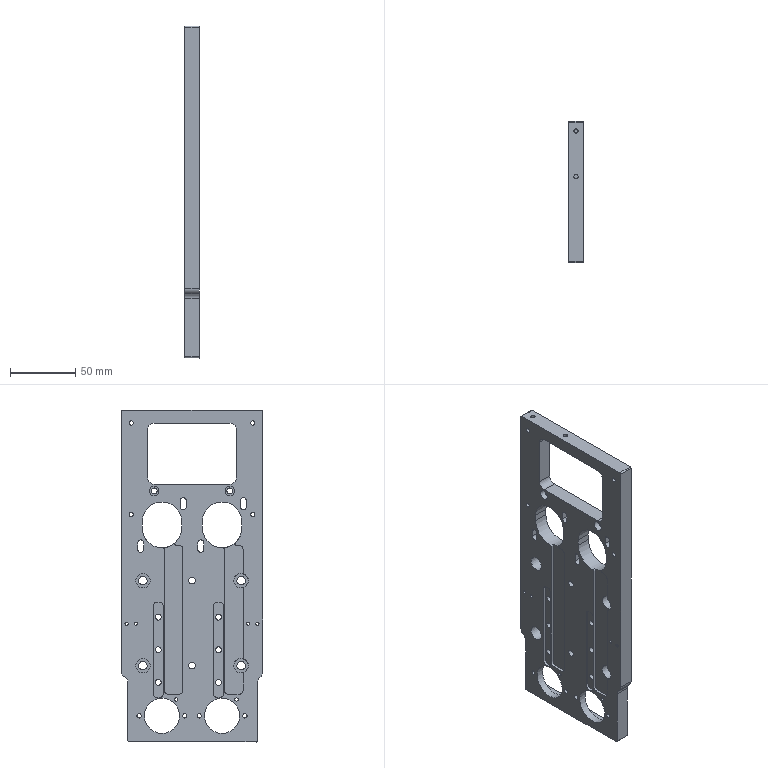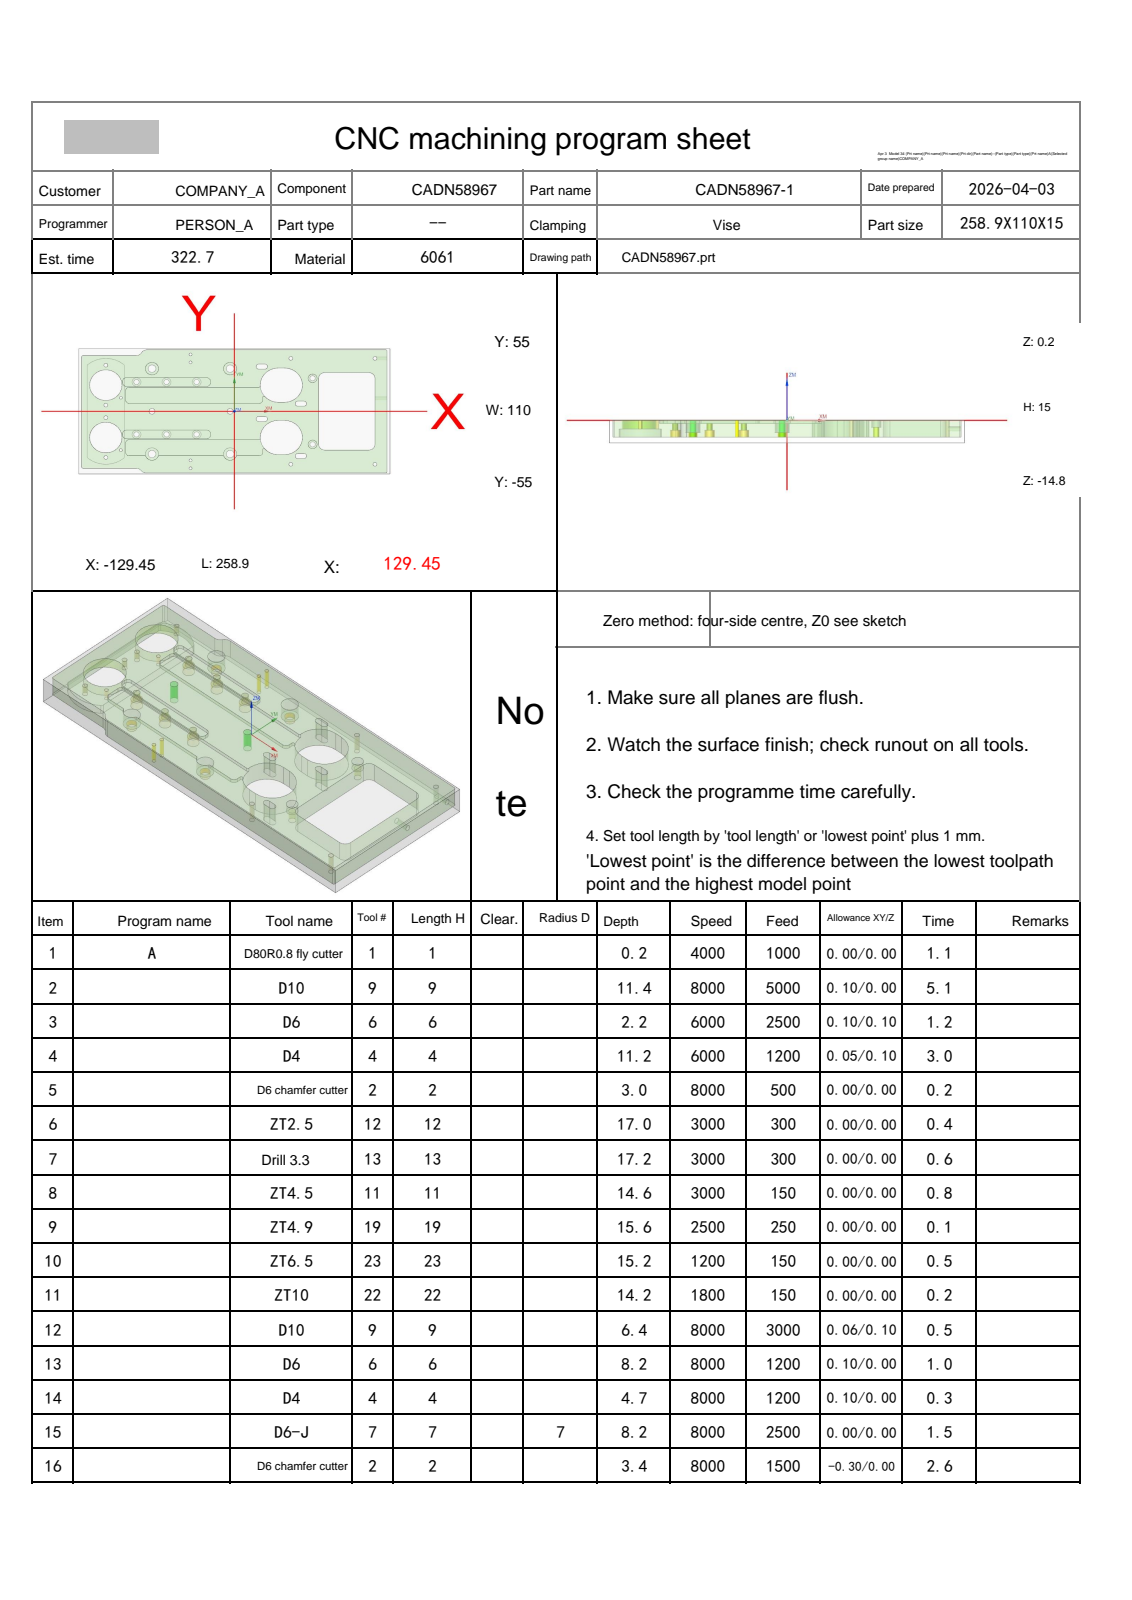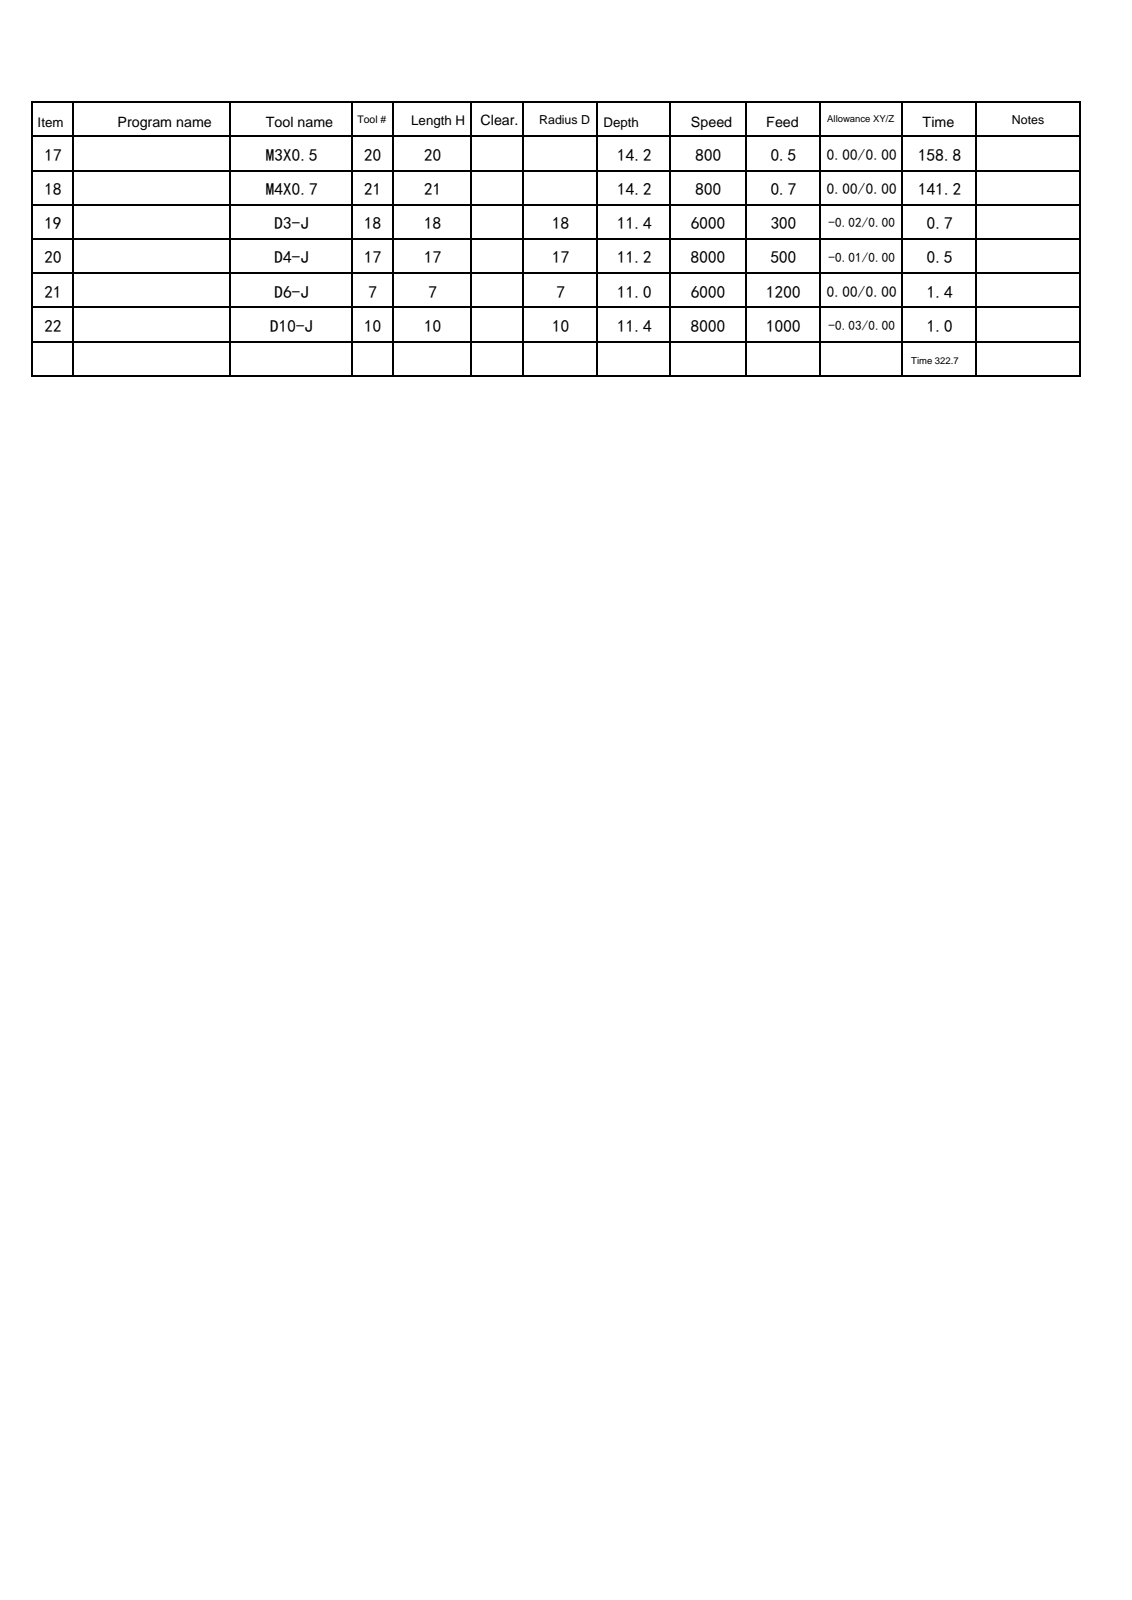NC program | NX | posted by the shop | part box 11 x 108 x 253.9 mm
Lines 3590 to 4069 of 8037:
N5 T02 M06
(D6 chamfer cutter  D=6. R=0. H=02 ce=0.00 di=0.10)
G00 G90 G54 X116.95 Y-46.5 M03 S8000
G43 H02 Z20.
M08
G98 G81 X116.95 Y-46.5 Z-.8 R1. F500.
X65.05 Y-29.
X46.95 Y-46.5
X-3.55 Y-37.5
Y0.0
X-31.45 Y-20.25 Z-2.8 R-1.
X-36.45 Y-43. Z-.8 R1.
Y-50.
X-68.55 Y-37.5
X-56.45 Y-20.25 Z-2.8 R-1.
X-68.55 Y0.0 Z-.8 R1.
X-81.45 Y-20.25 Z-2.8 R-1.
X-94.45 Y-34.045 Z-.8 R1.
X-106.95 Y-40.5
Y-23.
Y-5.5
Y5.5
X-94.45 Y11.955
X-106.95 Y23.
Y40.5
X-81.45 Y25.75 Z-2.8 R-1.
X-68.55 Y37.5 Z-.8 R1.
X-56.45 Y25.75 Z-2.8 R-1.
X-31.45
X-36.45 Y43. Z-.8 R1.
Y50.
X-3.55 Y37.5
X46.95 Y46.5
X65.05 Y29.
X116.95 Y46.5
G80
G00 Z20.
G91 G28 Z0.0
M05
M09
G91 G28 Z0.0
M01
N6 T12 M06
(ZT2.5 D=2.5 DR_a=118 H=12)
G00 G90 G54 X-36.45 Y-50. M03 S3000
G43 H12 Z20.
M08
G98 G83 X-36.45 Y-50. Z-16.751 R1. F300. Q2.
Y-43.
G98 G83 X-94.45 Y-34.045 Z-11.451 R1. Q2.
Y11.955
G98 G83 X-36.45 Y43. Z-16.751 R1. Q2.
Y50.
G80
G00 Z20.
G91 G28 Z0.0
M05
M09
G91 G28 Z0.0
M01
N7 T13 M06
(drill 3.3 D=3.3 DR_a=118 H=13)
G00 G90 G54 X-106.95 Y-40.5 M03 S3000
G43 H13 Z20.
M08
G98 G83 X-106.95 Y-40.5 Z-11.691 R1. F300. Q2.
Y-5.5
Y5.5
Y40.5
G98 G83 X46.95 Y46.5 Z-16.991 R1. Q2.
Y-46.5
X116.95
G80
G00 Z20.
G00 G90 X116.95 Y46.5 M03 S3000
Z20.
G98 G83 X116.95 Y46.5 Z-17. R1. F100. Q2.
G80
G00 Z20.
G91 G28 Z0.0
M05
M09
G91 G28 Z0.0
M01
N8 T11 M06
(ZT4.5 D=4.5 DR_a=118 H=11)
G00 G90 G54 X-81.45 Y-20.25 M03 S3000
G43 H11 Z20.
M08
G98 G83 X-81.45 Y-20.25 Z-9.852 R1. F150. Q3.
X-56.45
X-31.45
Y25.75
X-56.45
X-81.45
G80
G00 Z20.
G00 G90 X65.05 Y-29. M03 S2800
Z20.
G98 G83 X65.05 Y-29. Z-14.352 R1. F100. Q2.
Y29.
G80
G00 Z20.
G91 G28 Z0.0
M05
M09
G91 G28 Z0.0
M01
N9 T19 M06
(ZT4.9 D=4.9 DR_a=120 H=19)
G00 G90 G54 X-68.55 Y0.0 M03 S2500
G43 H19 Z20.
M08
G98 G83 X-68.55 Y0.0 Z-15.415 R1. F250. Q2.
X-3.55
G80
G00 Z20.
G91 G28 Z0.0
M05
M09
G91 G28 Z0.0
M01
N10 T23 M06
(ZT6.5 D=6.5 DR_a=118 H=23)
G00 G90 G54 X-68.55 Y-37.5 M03 S1200
G43 H23 Z20.
M08
G98 G83 X-68.55 Y-37.5 Z-14.953 R1. F150. Q2.
X-3.55
G98 G83 X-3.55 Y37.5 Z-14.953 R1. Q2.
X-68.55
G80
G00 Z20.
G91 G28 Z0.0
M05
M09
G91 G28 Z0.0
M01
N11 T22 M06
(ZT10 D=10. DR_a=118 H=22)
G00 G90 G54 X-106.95 Y-23. M03 S1800
G43 H22 Z20.
M08
G98 G83 X-106.95 Y-23. Z-14. R1. F150. Q3.
Y23.
G80
G00 Z20.
G91 G28 Z0.0
M05
M09
G91 G28 Z0.0
M01
N12 T09 M06
(D10  D=10. R=0. H=09 ce=0.06 di=0.10)
G00 G90 G54 X-101.614 Y-16.495 M03 S8000
G43 H09 Z20.
M08
Z1.
G01 X-102.511 Y-15.786 Z.94 F3000.
X-104.302 Y-14.954 Z.837
X-106.238 Y-14.56 Z.733
X-106.95 Z.696
X-107.662 Z.658
X-109.598 Y-14.954 Z.555
X-111.389 Y-15.786 Z.451
X-112.939 Y-17.011 Z.348
X-114.164 Y-18.561 Z.244
X-114.996 Y-20.352 Z.141
X-115.39 Y-22.288 Z.037
Y-23. Z0.0
G03 X-106.95 Y-31.44 Z-.141 I8.44 J0.0
X-98.51 Y-23. Z-.282 I0.0 J8.44
X-106.95 Y-14.56 Z-.423 I-8.44 J0.0
X-115.39 Y-23. Z-.564 I0.0 J-8.44
X-106.95 Y-31.44 Z-.705 I8.44 J0.0
X-98.51 Y-23. Z-.845 I0.0 J8.44
X-106.95 Y-14.56 Z-.986 I-8.44 J0.0
X-115.39 Y-23. Z-1.127 I0.0 J-8.44
X-106.95 Y-31.44 Z-1.268 I8.44 J0.0
X-98.51 Y-23. Z-1.409 I0.0 J8.44
X-106.95 Y-14.56 Z-1.55 I-8.44 J0.0
X-115.39 Y-23. Z-1.691 I0.0 J-8.44
X-106.95 Y-31.44 Z-1.832 I8.44 J0.0
X-98.51 Y-23. Z-1.973 I0.0 J8.44
X-106.95 Y-14.56 Z-2.114 I-8.44 J0.0
X-115.39 Y-23. Z-2.255 I0.0 J-8.44
X-106.95 Y-31.44 Z-2.395 I8.44 J0.0
X-98.51 Y-23. Z-2.536 I0.0 J8.44
X-106.95 Y-14.56 Z-2.677 I-8.44 J0.0
X-115.39 Y-23. Z-2.818 I0.0 J-8.44
X-106.95 Y-31.44 Z-2.959 I8.44 J0.0
X-98.51 Y-23. Z-3.1 I0.0 J8.44
X-106.95 Y-14.56 Z-3.241 I-8.44 J0.0
X-115.39 Y-23. Z-3.382 I0.0 J-8.44
X-106.95 Y-31.44 Z-3.523 I8.44 J0.0
X-98.51 Y-23. Z-3.664 I0.0 J8.44
X-106.95 Y-14.56 Z-3.805 I-8.44 J0.0
X-115.39 Y-23. Z-3.945 I0.0 J-8.44
X-106.95 Y-31.44 Z-4.086 I8.44 J0.0
X-98.51 Y-23. Z-4.227 I0.0 J8.44
X-106.95 Y-14.56 Z-4.368 I-8.44 J0.0
X-115.39 Y-23. Z-4.509 I0.0 J-8.44
X-106.95 Y-31.44 Z-4.65 I8.44 J0.0
X-98.51 Y-23. Z-4.791 I0.0 J8.44
X-106.95 Y-14.56 Z-4.932 I-8.44 J0.0
X-115.39 Y-23. Z-5.073 I0.0 J-8.44
X-106.95 Y-31.44 Z-5.214 I8.44 J0.0
X-98.51 Y-23. Z-5.355 I0.0 J8.44
X-106.95 Y-14.56 Z-5.495 I-8.44 J0.0
X-115.39 Y-23. Z-5.636 I0.0 J-8.44
X-106.95 Y-31.44 Z-5.777 I8.44 J0.0
X-98.51 Y-23. Z-5.918 I0.0 J8.44
X-106.95 Y-14.56 Z-6.059 I-8.44 J0.0
X-115.39 Y-23. Z-6.2 I0.0 J-8.44
X-106.95 Y-31.44 I8.44 J0.0
X-98.51 Y-23. I0.0 J8.44
X-106.95 Y-14.56 I-8.44 J0.0
X-115.39 Y-23. I0.0 J-8.44
X-115.381 Y-23.4 I8.44 J0.0
G01 Z-5.2
G00 Z20.
X-101.614 Y29.505
Z1.
G01 X-102.511 Y30.214 Z.94
X-104.302 Y31.046 Z.837
X-106.238 Y31.44 Z.733
X-107.662 Z.658
X-109.598 Y31.046 Z.555
X-111.389 Y30.214 Z.451
X-112.939 Y28.989 Z.348
X-114.164 Y27.439 Z.244
X-114.996 Y25.648 Z.141
X-115.39 Y23.712 Z.037
Y23. Z0.0
G03 X-106.95 Y14.56 Z-.141 I8.44 J0.0
X-98.51 Y23. Z-.282 I0.0 J8.44
X-106.95 Y31.44 Z-.423 I-8.44 J0.0
X-115.39 Y23. Z-.564 I0.0 J-8.44
X-106.95 Y14.56 Z-.705 I8.44 J0.0
X-98.51 Y23. Z-.845 I0.0 J8.44
X-106.95 Y31.44 Z-.986 I-8.44 J0.0
X-115.39 Y23. Z-1.127 I0.0 J-8.44
X-106.95 Y14.56 Z-1.268 I8.44 J0.0
X-98.51 Y23. Z-1.409 I0.0 J8.44
X-106.95 Y31.44 Z-1.55 I-8.44 J0.0
X-115.39 Y23. Z-1.691 I0.0 J-8.44
X-106.95 Y14.56 Z-1.832 I8.44 J0.0
X-98.51 Y23. Z-1.973 I0.0 J8.44
X-106.95 Y31.44 Z-2.114 I-8.44 J0.0
X-115.39 Y23. Z-2.255 I0.0 J-8.44
X-106.95 Y14.56 Z-2.395 I8.44 J0.0
X-98.51 Y23. Z-2.536 I0.0 J8.44
X-106.95 Y31.44 Z-2.677 I-8.44 J0.0
X-115.39 Y23. Z-2.818 I0.0 J-8.44
X-106.95 Y14.56 Z-2.959 I8.44 J0.0
X-98.51 Y23. Z-3.1 I0.0 J8.44
X-106.95 Y31.44 Z-3.241 I-8.44 J0.0
X-115.39 Y23. Z-3.382 I0.0 J-8.44
X-106.95 Y14.56 Z-3.523 I8.44 J0.0
X-98.51 Y23. Z-3.664 I0.0 J8.44
X-106.95 Y31.44 Z-3.805 I-8.44 J0.0
X-115.39 Y23. Z-3.945 I0.0 J-8.44
X-106.95 Y14.56 Z-4.086 I8.44 J0.0
X-98.51 Y23. Z-4.227 I0.0 J8.44
X-106.95 Y31.44 Z-4.368 I-8.44 J0.0
X-115.39 Y23. Z-4.509 I0.0 J-8.44
X-106.95 Y14.56 Z-4.65 I8.44 J0.0
X-98.51 Y23. Z-4.791 I0.0 J8.44
X-106.95 Y31.44 Z-4.932 I-8.44 J0.0
X-115.39 Y23. Z-5.073 I0.0 J-8.44
X-106.95 Y14.56 Z-5.214 I8.44 J0.0
X-98.51 Y23. Z-5.355 I0.0 J8.44
X-106.95 Y31.44 Z-5.495 I-8.44 J0.0
X-115.39 Y23. Z-5.636 I0.0 J-8.44
X-106.95 Y14.56 Z-5.777 I8.44 J0.0
X-98.51 Y23. Z-5.918 I0.0 J8.44
X-106.95 Y31.44 Z-6.059 I-8.44 J0.0
X-115.39 Y23. Z-6.2 I0.0 J-8.44
X-106.95 Y14.56 I8.44 J0.0
X-98.51 Y23. I0.0 J8.44
X-106.95 Y31.44 I-8.44 J0.0
X-115.39 Y23. I0.0 J-8.44
X-115.381 Y22.6 I8.44 J0.0
G01 Z-5.2
G00 Z20.
G91 G28 Z0.0
M05
M09
G91 G28 Z0.0
M01
N13 T06 M06
(D6  D=6. R=0. H=06 ce=0.10 di=0.00)
G00 G90 G54 X-3.55 Y-37.5 M03 S8000
G43 H06 Z20.
M08
Z.5
G03 X-2.35 Y-36.3 I0.0 J1.2 F1200.
X-3.55 Y-35.1 I-1.2 J0.0
X-3.55 Y-35.1 Z0.0 I0.0 J-2.4
X-3.55 Y-35.1 Z-.5 I0.0 J-2.4
X-3.55 Y-35.1 Z-1. I0.0 J-2.4
X-3.55 Y-35.1 Z-1.5 I0.0 J-2.4
X-3.55 Y-35.1 Z-2. I0.0 J-2.4
X-3.55 Y-35.1 Z-2.5 I0.0 J-2.4
X-3.55 Y-35.1 Z-3. I0.0 J-2.4
X-3.55 Y-35.1 Z-3.5 I0.0 J-2.4
X-3.55 Y-35.1 Z-4. I0.0 J-2.4
X-3.55 Y-35.1 Z-4.5 I0.0 J-2.4
X-3.55 Y-35.1 Z-5. I0.0 J-2.4
X-3.55 Y-35.1 Z-5.5 I0.0 J-2.4
X-3.55 Y-35.1 Z-6. I0.0 J-2.4
X-3.55 Y-35.1 Z-6.5 I0.0 J-2.4
X-3.55 Y-35.1 Z-7. I0.0 J-2.4
X-3.55 Y-35.1 Z-7.5 I0.0 J-2.4
X-3.55 Y-35.1 Z-8. I0.0 J-2.4
X-5.95 Y-37.5 I0.0 J-2.4
X-3.55 Y-39.9 I2.4 J0.0
X-1.15 Y-37.5 I0.0 J2.4
X-3.55 Y-35.1 I-2.4 J0.0
X-4.75 Y-36.3 I0.0 J-1.2
X-3.55 Y-37.5 I1.2 J0.0
G00 Z20.
X-68.55
Z.5
G03 X-67.35 Y-36.3 I0.0 J1.2
X-68.55 Y-35.1 I-1.2 J0.0
X-68.55 Y-35.1 Z0.0 I0.0 J-2.4
X-68.55 Y-35.1 Z-.5 I0.0 J-2.4
X-68.55 Y-35.1 Z-1. I0.0 J-2.4
X-68.55 Y-35.1 Z-1.5 I0.0 J-2.4
X-68.55 Y-35.1 Z-2. I0.0 J-2.4
X-68.55 Y-35.1 Z-2.5 I0.0 J-2.4
X-68.55 Y-35.1 Z-3. I0.0 J-2.4
X-68.55 Y-35.1 Z-3.5 I0.0 J-2.4
X-68.55 Y-35.1 Z-4. I0.0 J-2.4
X-68.55 Y-35.1 Z-4.5 I0.0 J-2.4
X-68.55 Y-35.1 Z-5. I0.0 J-2.4
X-68.55 Y-35.1 Z-5.5 I0.0 J-2.4
X-68.55 Y-35.1 Z-6. I0.0 J-2.4
X-68.55 Y-35.1 Z-6.5 I0.0 J-2.4
X-68.55 Y-35.1 Z-7. I0.0 J-2.4
X-68.55 Y-35.1 Z-7.5 I0.0 J-2.4
X-68.55 Y-35.1 Z-8. I0.0 J-2.4
X-70.95 Y-37.5 I0.0 J-2.4
X-68.55 Y-39.9 I2.4 J0.0
X-66.15 Y-37.5 I0.0 J2.4
X-68.55 Y-35.1 I-2.4 J0.0
X-69.75 Y-36.3 I0.0 J-1.2
X-68.55 Y-37.5 I1.2 J0.0
G00 Z20.
Y37.5
Z.5
G03 X-67.35 Y38.7 I0.0 J1.2
X-68.55 Y39.9 I-1.2 J0.0
X-68.55 Y39.9 Z0.0 I0.0 J-2.4
X-68.55 Y39.9 Z-.5 I0.0 J-2.4
X-68.55 Y39.9 Z-1. I0.0 J-2.4
X-68.55 Y39.9 Z-1.5 I0.0 J-2.4
X-68.55 Y39.9 Z-2. I0.0 J-2.4
X-68.55 Y39.9 Z-2.5 I0.0 J-2.4
X-68.55 Y39.9 Z-3. I0.0 J-2.4
X-68.55 Y39.9 Z-3.5 I0.0 J-2.4
X-68.55 Y39.9 Z-4. I0.0 J-2.4
X-68.55 Y39.9 Z-4.5 I0.0 J-2.4
X-68.55 Y39.9 Z-5. I0.0 J-2.4
X-68.55 Y39.9 Z-5.5 I0.0 J-2.4
X-68.55 Y39.9 Z-6. I0.0 J-2.4
X-68.55 Y39.9 Z-6.5 I0.0 J-2.4
X-68.55 Y39.9 Z-7. I0.0 J-2.4
X-68.55 Y39.9 Z-7.5 I0.0 J-2.4
X-68.55 Y39.9 Z-8. I0.0 J-2.4
X-70.95 Y37.5 I0.0 J-2.4
X-68.55 Y35.1 I2.4 J0.0
X-66.15 Y37.5 I0.0 J2.4
X-68.55 Y39.9 I-2.4 J0.0
X-69.75 Y38.7 I0.0 J-1.2
X-68.55 Y37.5 I1.2 J0.0
G00 Z20.
X-3.55
Z.5
G03 X-2.35 Y38.7 I0.0 J1.2
X-3.55 Y39.9 I-1.2 J0.0
X-3.55 Y39.9 Z0.0 I0.0 J-2.4
X-3.55 Y39.9 Z-.5 I0.0 J-2.4
X-3.55 Y39.9 Z-1. I0.0 J-2.4
X-3.55 Y39.9 Z-1.5 I0.0 J-2.4
X-3.55 Y39.9 Z-2. I0.0 J-2.4
X-3.55 Y39.9 Z-2.5 I0.0 J-2.4
X-3.55 Y39.9 Z-3. I0.0 J-2.4
X-3.55 Y39.9 Z-3.5 I0.0 J-2.4
X-3.55 Y39.9 Z-4. I0.0 J-2.4
X-3.55 Y39.9 Z-4.5 I0.0 J-2.4
X-3.55 Y39.9 Z-5. I0.0 J-2.4
X-3.55 Y39.9 Z-5.5 I0.0 J-2.4
X-3.55 Y39.9 Z-6. I0.0 J-2.4
X-3.55 Y39.9 Z-6.5 I0.0 J-2.4
X-3.55 Y39.9 Z-7. I0.0 J-2.4
X-3.55 Y39.9 Z-7.5 I0.0 J-2.4
X-3.55 Y39.9 Z-8. I0.0 J-2.4
X-5.95 Y37.5 I0.0 J-2.4
X-3.55 Y35.1 I2.4 J0.0
X-1.15 Y37.5 I0.0 J2.4
X-3.55 Y39.9 I-2.4 J0.0
X-4.75 Y38.7 I0.0 J-1.2
X-3.55 Y37.5 I1.2 J0.0
G00 Z20.
G91 G28 Z0.0
M05
M09
G91 G28 Z0.0
M01
N14 T04 M06
(D4  D=4. R=0. H=04 ce=0.10 di=0.00)
G00 G90 G54 X65.05 Y-29. M03 S8000
G43 H04 Z20.
M08
Z.5
G03 X65.875 Y-28.175 I0.0 J.825 F1200.
X65.05 Y-27.35 I-.825 J0.0
X65.05 Y-27.35 Z.2 I0.0 J-1.65
X65.05 Y-27.35 Z-.1 I0.0 J-1.65
X65.05 Y-27.35 Z-.4 I0.0 J-1.65
X65.05 Y-27.35 Z-.7 I0.0 J-1.65
X65.05 Y-27.35 Z-1. I0.0 J-1.65
X65.05 Y-27.35 Z-1.3 I0.0 J-1.65
X65.05 Y-27.35 Z-1.6 I0.0 J-1.65
X65.05 Y-27.35 Z-1.9 I0.0 J-1.65
X65.05 Y-27.35 Z-2.2 I0.0 J-1.65
X65.05 Y-27.35 Z-2.5 I0.0 J-1.65
X65.05 Y-27.35 Z-2.8 I0.0 J-1.65
X65.05 Y-27.35 Z-3.1 I0.0 J-1.65
X65.05 Y-27.35 Z-3.4 I0.0 J-1.65
X65.05 Y-27.35 Z-3.7 I0.0 J-1.65
X65.05 Y-27.35 Z-4. I0.0 J-1.65
X65.05 Y-27.35 Z-4.3 I0.0 J-1.65
X66.479 Y-29.825 Z-4.5 I0.0 J-1.65
X66.7 Y-29. I-1.429 J.825
X65.05 Y-27.35 I-1.65 J0.0
X63.4 Y-29. I0.0 J-1.65
X65.05 Y-30.65 I1.65 J0.0
X66.479 Y-29.825 I0.0 J1.65
X66.589 Y-29.413 I-.714 J.413
X65.764 Y-28.588 I-.825 J0.0
X65.05 Y-29. I0.0 J-.825
G00 Z20.
Y29.
Z.5
G03 X65.875 Y29.825 I0.0 J.825
X65.05 Y30.65 I-.825 J0.0
X65.05 Y30.65 Z.2 I0.0 J-1.65
X65.05 Y30.65 Z-.1 I0.0 J-1.65
X65.05 Y30.65 Z-.4 I0.0 J-1.65
X65.05 Y30.65 Z-.7 I0.0 J-1.65
X65.05 Y30.65 Z-1. I0.0 J-1.65
X65.05 Y30.65 Z-1.3 I0.0 J-1.65
X65.05 Y30.65 Z-1.6 I0.0 J-1.65
X65.05 Y30.65 Z-1.9 I0.0 J-1.65
X65.05 Y30.65 Z-2.2 I0.0 J-1.65
X65.05 Y30.65 Z-2.5 I0.0 J-1.65
X65.05 Y30.65 Z-2.8 I0.0 J-1.65
X65.05 Y30.65 Z-3.1 I0.0 J-1.65
X65.05 Y30.65 Z-3.4 I0.0 J-1.65
X65.05 Y30.65 Z-3.7 I0.0 J-1.65
X65.05 Y30.65 Z-4. I0.0 J-1.65
X65.05 Y30.65 Z-4.3 I0.0 J-1.65
X66.479 Y28.175 Z-4.5 I0.0 J-1.65
X66.7 Y29. I-1.429 J.825
X65.05 Y30.65 I-1.65 J0.0
X63.4 Y29. I0.0 J-1.65
X65.05 Y27.35 I1.65 J0.0
X66.479 Y28.175 I0.0 J1.65
X66.589 Y28.587 I-.714 J.413
X65.764 Y29.412 I-.825 J0.0
X65.05 Y29. I0.0 J-.825
G00 Z20.
G91 G28 Z0.0
M05
M09
G91 G28 Z0.0
M01